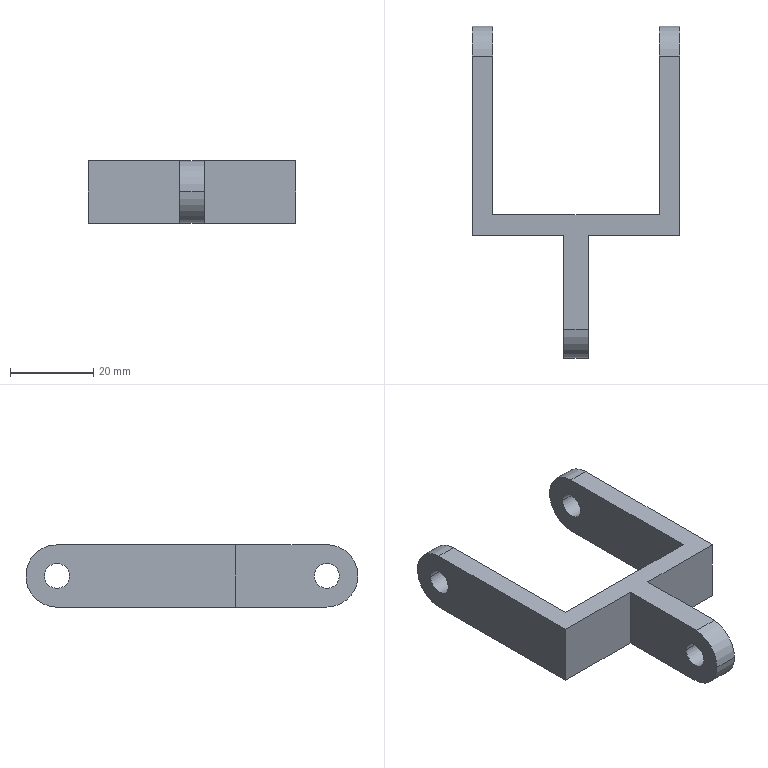Part | SolidWorks | features Extrusion 1, ICE 1 | 1 solid | 24 faces | box 50 x 80 x 15 mm | volume 12391 mm3 | plane 14 | cylinder 10 | commonest cylinder face diameters 6 x6 15 x4
STEP:
#1=CARTESIAN_POINT('',(25.,76.,7.503));
#2=VERTEX_POINT('',#1);
#3=CARTESIAN_POINT('',(25.,70.,7.503));
#4=VERTEX_POINT('',#3);
#5=CARTESIAN_POINT('',(25.,73.,7.503));
#6=DIRECTION('',(-1.,0.,0.));
#7=DIRECTION('',(0.,-1.,0.));
#8=AXIS2_PLACEMENT_3D('',#5,#6,#7);
#9=CIRCLE('',#8,3.);
#10=EDGE_CURVE('',#2,#4,#9,.T.);
#11=ORIENTED_EDGE('',*,*,#10,.F.);
#12=CARTESIAN_POINT('',(20.,76.,7.503));
#13=VERTEX_POINT('',#12);
#14=CARTESIAN_POINT('',(25.,76.,7.503));
#15=DIRECTION('',(-1.,0.,0.));
#16=VECTOR('',#15,1000.);
#17=LINE('',#14,#16);
#18=EDGE_CURVE('',#2,#13,#17,.T.);
#19=ORIENTED_EDGE('',*,*,#18,.T.);
#20=CARTESIAN_POINT('',(20.,70.,7.503));
#21=VERTEX_POINT('',#20);
#22=CARTESIAN_POINT('',(20.,73.,7.503));
#23=DIRECTION('',(1.,0.,0.));
#24=DIRECTION('',(0.,0.,-1.));
#25=AXIS2_PLACEMENT_3D('',#22,#23,#24);
#26=CIRCLE('',#25,3.);
#27=EDGE_CURVE('',#21,#13,#26,.T.);
#28=ORIENTED_EDGE('',*,*,#27,.F.);
#29=CARTESIAN_POINT('',(25.,70.,7.503));
#30=DIRECTION('',(-1.,0.,0.));
#31=VECTOR('',#30,1000.);
#32=LINE('',#29,#31);
#33=EDGE_CURVE('',#4,#21,#32,.T.);
#34=ORIENTED_EDGE('',*,*,#33,.F.);
#35=EDGE_LOOP('',(#11,#19,#28,#34));
#36=FACE_OUTER_BOUND('',#35,.T.);
#37=CARTESIAN_POINT('',(25.,73.,7.503));
#38=DIRECTION('',(-1.,0.,0.));
#39=DIRECTION('',(0.,-1.,0.));
#40=AXIS2_PLACEMENT_3D('',#37,#38,#39);
#41=CYLINDRICAL_SURFACE('',#40,3.);
#42=ADVANCED_FACE('',(#36),#41,.F.);
#43=CARTESIAN_POINT('',(-20.,76.,7.503));
#44=VERTEX_POINT('',#43);
#45=CARTESIAN_POINT('',(-20.,70.,7.503));
#46=VERTEX_POINT('',#45);
#47=CARTESIAN_POINT('',(-20.,73.,7.503));
#48=DIRECTION('',(-1.,0.,0.));
#49=DIRECTION('',(0.,0.,1.));
#50=AXIS2_PLACEMENT_3D('',#47,#48,#49);
#51=CIRCLE('',#50,3.);
#52=EDGE_CURVE('',#44,#46,#51,.T.);
#53=ORIENTED_EDGE('',*,*,#52,.F.);
#54=CARTESIAN_POINT('',(-25.,76.,7.503));
#55=VERTEX_POINT('',#54);
#56=CARTESIAN_POINT('',(25.,76.,7.503));
#57=DIRECTION('',(-1.,0.,0.));
#58=VECTOR('',#57,1000.);
#59=LINE('',#56,#58);
#60=EDGE_CURVE('',#44,#55,#59,.T.);
#61=ORIENTED_EDGE('',*,*,#60,.T.);
#62=CARTESIAN_POINT('',(-25.,70.,7.503));
#63=VERTEX_POINT('',#62);
#64=CARTESIAN_POINT('',(-25.,73.,7.503));
#65=DIRECTION('',(-1.,0.,0.));
#66=DIRECTION('',(0.,-1.,0.));
#67=AXIS2_PLACEMENT_3D('',#64,#65,#66);
#68=CIRCLE('',#67,3.);
#69=EDGE_CURVE('',#55,#63,#68,.T.);
#70=ORIENTED_EDGE('',*,*,#69,.T.);
#71=CARTESIAN_POINT('',(25.,70.,7.503));
#72=DIRECTION('',(-1.,0.,0.));
#73=VECTOR('',#72,1000.);
#74=LINE('',#71,#73);
#75=EDGE_CURVE('',#46,#63,#74,.T.);
#76=ORIENTED_EDGE('',*,*,#75,.F.);
#77=EDGE_LOOP('',(#53,#61,#70,#76));
#78=FACE_OUTER_BOUND('',#77,.T.);
#79=CARTESIAN_POINT('',(25.,73.,7.503));
#80=DIRECTION('',(-1.,0.,0.));
#81=DIRECTION('',(0.,-1.,0.));
#82=AXIS2_PLACEMENT_3D('',#79,#80,#81);
#83=CYLINDRICAL_SURFACE('',#82,3.);
#84=ADVANCED_FACE('',(#78),#83,.F.);
#85=CARTESIAN_POINT('',(3.,11.,7.524));
#86=VERTEX_POINT('',#85);
#87=CARTESIAN_POINT('',(3.,5.,7.524));
#88=VERTEX_POINT('',#87);
#89=CARTESIAN_POINT('',(3.,8.,7.524));
#90=DIRECTION('',(-1.,0.,0.));
#91=DIRECTION('',(0.,-1.,0.));
#92=AXIS2_PLACEMENT_3D('',#89,#90,#91);
#93=CIRCLE('',#92,3.);
#94=EDGE_CURVE('',#86,#88,#93,.T.);
#95=ORIENTED_EDGE('',*,*,#94,.F.);
#96=CARTESIAN_POINT('',(-3.,11.,7.524));
#97=VERTEX_POINT('',#96);
#98=CARTESIAN_POINT('',(25.,11.,7.524));
#99=DIRECTION('',(-1.,0.,0.));
#100=VECTOR('',#99,1000.);
#101=LINE('',#98,#100);
#102=EDGE_CURVE('',#86,#97,#101,.T.);
#103=ORIENTED_EDGE('',*,*,#102,.T.);
#104=CARTESIAN_POINT('',(-3.,5.,7.524));
#105=VERTEX_POINT('',#104);
#106=CARTESIAN_POINT('',(-3.,8.,7.524));
#107=DIRECTION('',(1.,0.,0.));
#108=DIRECTION('',(0.,1.,0.));
#109=AXIS2_PLACEMENT_3D('',#106,#107,#108);
#110=CIRCLE('',#109,3.);
#111=EDGE_CURVE('',#105,#97,#110,.T.);
#112=ORIENTED_EDGE('',*,*,#111,.F.);
#113=CARTESIAN_POINT('',(25.,5.,7.524));
#114=DIRECTION('',(-1.,0.,0.));
#115=VECTOR('',#114,1000.);
#116=LINE('',#113,#115);
#117=EDGE_CURVE('',#88,#105,#116,.T.);
#118=ORIENTED_EDGE('',*,*,#117,.F.);
#119=EDGE_LOOP('',(#95,#103,#112,#118));
#120=FACE_OUTER_BOUND('',#119,.T.);
#121=CARTESIAN_POINT('',(25.,8.,7.524));
#122=DIRECTION('',(-1.,0.,0.));
#123=DIRECTION('',(0.,-1.,0.));
#124=AXIS2_PLACEMENT_3D('',#121,#122,#123);
#125=CYLINDRICAL_SURFACE('',#124,3.);
#126=ADVANCED_FACE('',(#120),#125,.F.);
#127=CARTESIAN_POINT('',(3.,0.5,7.524));
#128=VERTEX_POINT('',#127);
#129=CARTESIAN_POINT('',(3.,8.,0.02363));
#130=VERTEX_POINT('',#129);
#131=CARTESIAN_POINT('',(3.,8.,7.524));
#132=DIRECTION('',(1.,0.,0.));
#133=DIRECTION('',(0.,-1.,0.));
#134=AXIS2_PLACEMENT_3D('',#131,#132,#133);
#135=CIRCLE('',#134,7.5);
#136=EDGE_CURVE('',#128,#130,#135,.T.);
#137=ORIENTED_EDGE('',*,*,#136,.F.);
#138=CARTESIAN_POINT('',(-3.,0.5,7.524));
#139=VERTEX_POINT('',#138);
#140=CARTESIAN_POINT('',(25.,0.5,7.524));
#141=DIRECTION('',(-1.,0.,0.));
#142=VECTOR('',#141,1000.);
#143=LINE('',#140,#142);
#144=EDGE_CURVE('',#128,#139,#143,.T.);
#145=ORIENTED_EDGE('',*,*,#144,.T.);
#146=CARTESIAN_POINT('',(-3.,8.,0.02363));
#147=VERTEX_POINT('',#146);
#148=CARTESIAN_POINT('',(-3.,8.,7.524));
#149=DIRECTION('',(-1.,0.,0.));
#150=DIRECTION('',(0.,1.,0.));
#151=AXIS2_PLACEMENT_3D('',#148,#149,#150);
#152=CIRCLE('',#151,7.5);
#153=EDGE_CURVE('',#147,#139,#152,.T.);
#154=ORIENTED_EDGE('',*,*,#153,.F.);
#155=CARTESIAN_POINT('',(25.,8.,0.02363));
#156=DIRECTION('',(-1.,0.,0.));
#157=VECTOR('',#156,1000.);
#158=LINE('',#155,#157);
#159=EDGE_CURVE('',#130,#147,#158,.T.);
#160=ORIENTED_EDGE('',*,*,#159,.F.);
#161=EDGE_LOOP('',(#137,#145,#154,#160));
#162=FACE_OUTER_BOUND('',#161,.T.);
#163=CARTESIAN_POINT('',(25.,8.,7.524));
#164=DIRECTION('',(-1.,0.,0.));
#165=DIRECTION('',(0.,-1.,0.));
#166=AXIS2_PLACEMENT_3D('',#163,#164,#165);
#167=CYLINDRICAL_SURFACE('',#166,7.5);
#168=ADVANCED_FACE('',(#162),#167,.T.);
#169=CARTESIAN_POINT('',(3.,8.,7.524));
#170=DIRECTION('',(-1.,0.,0.));
#171=DIRECTION('',(0.,-1.,0.));
#172=AXIS2_PLACEMENT_3D('',#169,#170,#171);
#173=CIRCLE('',#172,3.);
#174=EDGE_CURVE('',#88,#86,#173,.T.);
#175=ORIENTED_EDGE('',*,*,#174,.T.);
#176=ORIENTED_EDGE('',*,*,#94,.T.);
#177=EDGE_LOOP('',(#175,#176));
#178=FACE_BOUND('',#177,.T.);
#179=CARTESIAN_POINT('',(3.,7.405,15.));
#180=VERTEX_POINT('',#179);
#181=CARTESIAN_POINT('',(3.,30.,15.));
#182=VERTEX_POINT('',#181);
#183=CARTESIAN_POINT('',(3.,30.,15.));
#184=DIRECTION('',(0.,1.,0.));
#185=VECTOR('',#184,1000.);
#186=LINE('',#183,#185);
#187=EDGE_CURVE('',#180,#182,#186,.T.);
#188=ORIENTED_EDGE('',*,*,#187,.F.);
#189=CARTESIAN_POINT('',(3.,8.,7.524));
#190=DIRECTION('',(1.,0.,0.));
#191=DIRECTION('',(0.,-1.,0.));
#192=AXIS2_PLACEMENT_3D('',#189,#190,#191);
#193=CIRCLE('',#192,7.5);
#194=EDGE_CURVE('',#180,#128,#193,.T.);
#195=ORIENTED_EDGE('',*,*,#194,.T.);
#196=ORIENTED_EDGE('',*,*,#136,.T.);
#197=CARTESIAN_POINT('',(3.,7.989,0.));
#198=VERTEX_POINT('',#197);
#199=CARTESIAN_POINT('',(3.,18.014,20.782));
#200=DIRECTION('',(0.,-0.4345,-0.9007));
#201=VECTOR('',#200,1000.);
#202=LINE('',#199,#201);
#203=EDGE_CURVE('',#130,#198,#202,.T.);
#204=ORIENTED_EDGE('',*,*,#203,.T.);
#205=CARTESIAN_POINT('',(3.,30.,0.));
#206=VERTEX_POINT('',#205);
#207=CARTESIAN_POINT('',(3.,30.,0.));
#208=DIRECTION('',(0.,1.,0.));
#209=VECTOR('',#208,1000.);
#210=LINE('',#207,#209);
#211=EDGE_CURVE('',#198,#206,#210,.T.);
#212=ORIENTED_EDGE('',*,*,#211,.T.);
#213=CARTESIAN_POINT('',(3.,30.,15.));
#214=DIRECTION('',(0.,0.,-1.));
#215=VECTOR('',#214,1000.);
#216=LINE('',#213,#215);
#217=EDGE_CURVE('',#182,#206,#216,.T.);
#218=ORIENTED_EDGE('',*,*,#217,.F.);
#219=EDGE_LOOP('',(#188,#195,#196,#204,#212,#218));
#220=FACE_OUTER_BOUND('',#219,.T.);
#221=CARTESIAN_POINT('',(3.,30.,15.));
#222=DIRECTION('',(-1.,0.,0.));
#223=DIRECTION('',(0.,-1.,0.));
#224=AXIS2_PLACEMENT_3D('',#221,#222,#223);
#225=PLANE('',#224);
#226=ADVANCED_FACE('',(#178,#220),#225,.F.);
#227=CARTESIAN_POINT('',(25.,30.,0.));
#228=VERTEX_POINT('',#227);
#229=CARTESIAN_POINT('',(25.,30.,0.));
#230=DIRECTION('',(1.,0.,0.));
#231=VECTOR('',#230,1000.);
#232=LINE('',#229,#231);
#233=EDGE_CURVE('',#206,#228,#232,.T.);
#234=ORIENTED_EDGE('',*,*,#233,.T.);
#235=CARTESIAN_POINT('',(25.,30.,15.));
#236=VERTEX_POINT('',#235);
#237=CARTESIAN_POINT('',(25.,30.,15.));
#238=DIRECTION('',(0.,0.,-1.));
#239=VECTOR('',#238,1000.);
#240=LINE('',#237,#239);
#241=EDGE_CURVE('',#236,#228,#240,.T.);
#242=ORIENTED_EDGE('',*,*,#241,.F.);
#243=CARTESIAN_POINT('',(25.,30.,15.));
#244=DIRECTION('',(1.,0.,0.));
#245=VECTOR('',#244,1000.);
#246=LINE('',#243,#245);
#247=EDGE_CURVE('',#182,#236,#246,.T.);
#248=ORIENTED_EDGE('',*,*,#247,.F.);
#249=ORIENTED_EDGE('',*,*,#217,.T.);
#250=EDGE_LOOP('',(#234,#242,#248,#249));
#251=FACE_OUTER_BOUND('',#250,.T.);
#252=CARTESIAN_POINT('',(25.,30.,15.));
#253=DIRECTION('',(0.,1.,0.));
#254=DIRECTION('',(0.,0.,1.));
#255=AXIS2_PLACEMENT_3D('',#252,#253,#254);
#256=PLANE('',#255);
#257=ADVANCED_FACE('',(#251),#256,.F.);
#258=CARTESIAN_POINT('',(25.,73.,7.503));
#259=DIRECTION('',(-1.,0.,0.));
#260=DIRECTION('',(0.,-1.,0.));
#261=AXIS2_PLACEMENT_3D('',#258,#259,#260);
#262=CIRCLE('',#261,3.);
#263=EDGE_CURVE('',#4,#2,#262,.T.);
#264=ORIENTED_EDGE('',*,*,#263,.T.);
#265=ORIENTED_EDGE('',*,*,#10,.T.);
#266=EDGE_LOOP('',(#264,#265));
#267=FACE_BOUND('',#266,.T.);
#268=CARTESIAN_POINT('',(25.,73.001,0.));
#269=VERTEX_POINT('',#268);
#270=CARTESIAN_POINT('',(25.,73.,0.00323));
#271=VERTEX_POINT('',#270);
#272=CARTESIAN_POINT('',(25.,73.,0.00323));
#273=DIRECTION('',(0.,-0.159,0.9873));
#274=VECTOR('',#273,1000.);
#275=LINE('',#272,#274);
#276=EDGE_CURVE('',#269,#271,#275,.T.);
#277=ORIENTED_EDGE('',*,*,#276,.T.);
#278=CARTESIAN_POINT('',(25.,73.22,15.));
#279=VERTEX_POINT('',#278);
#280=CARTESIAN_POINT('',(25.,73.,7.503));
#281=DIRECTION('',(1.,0.,0.));
#282=DIRECTION('',(0.,-1.,0.));
#283=AXIS2_PLACEMENT_3D('',#280,#281,#282);
#284=CIRCLE('',#283,7.5);
#285=EDGE_CURVE('',#271,#279,#284,.T.);
#286=ORIENTED_EDGE('',*,*,#285,.T.);
#287=CARTESIAN_POINT('',(25.,85.,15.));
#288=DIRECTION('',(0.,1.,0.));
#289=VECTOR('',#288,1000.);
#290=LINE('',#287,#289);
#291=EDGE_CURVE('',#236,#279,#290,.T.);
#292=ORIENTED_EDGE('',*,*,#291,.F.);
#293=ORIENTED_EDGE('',*,*,#241,.T.);
#294=CARTESIAN_POINT('',(25.,85.,0.));
#295=DIRECTION('',(0.,1.,0.));
#296=VECTOR('',#295,1000.);
#297=LINE('',#294,#296);
#298=EDGE_CURVE('',#228,#269,#297,.T.);
#299=ORIENTED_EDGE('',*,*,#298,.T.);
#300=EDGE_LOOP('',(#277,#286,#292,#293,#299));
#301=FACE_OUTER_BOUND('',#300,.T.);
#302=CARTESIAN_POINT('',(25.,85.,15.));
#303=DIRECTION('',(-1.,0.,0.));
#304=DIRECTION('',(0.,-1.,0.));
#305=AXIS2_PLACEMENT_3D('',#302,#303,#304);
#306=PLANE('',#305);
#307=ADVANCED_FACE('',(#267,#301),#306,.F.);
#308=ORIENTED_EDGE('',*,*,#27,.T.);
#309=CARTESIAN_POINT('',(20.,73.,7.503));
#310=DIRECTION('',(1.,0.,0.));
#311=DIRECTION('',(0.,0.,-1.));
#312=AXIS2_PLACEMENT_3D('',#309,#310,#311);
#313=CIRCLE('',#312,3.);
#314=EDGE_CURVE('',#13,#21,#313,.T.);
#315=ORIENTED_EDGE('',*,*,#314,.T.);
#316=EDGE_LOOP('',(#308,#315));
#317=FACE_BOUND('',#316,.T.);
#318=CARTESIAN_POINT('',(20.,73.22,15.));
#319=VERTEX_POINT('',#318);
#320=CARTESIAN_POINT('',(20.,35.,15.));
#321=VERTEX_POINT('',#320);
#322=CARTESIAN_POINT('',(20.,35.,15.));
#323=DIRECTION('',(0.,-1.,0.));
#324=VECTOR('',#323,1000.);
#325=LINE('',#322,#324);
#326=EDGE_CURVE('',#319,#321,#325,.T.);
#327=ORIENTED_EDGE('',*,*,#326,.F.);
#328=CARTESIAN_POINT('',(20.,73.,0.00323));
#329=VERTEX_POINT('',#328);
#330=CARTESIAN_POINT('',(20.,73.,7.503));
#331=DIRECTION('',(-1.,0.,0.));
#332=DIRECTION('',(0.,0.,-1.));
#333=AXIS2_PLACEMENT_3D('',#330,#331,#332);
#334=CIRCLE('',#333,7.5);
#335=EDGE_CURVE('',#319,#329,#334,.T.);
#336=ORIENTED_EDGE('',*,*,#335,.T.);
#337=CARTESIAN_POINT('',(20.,73.001,0.));
#338=VERTEX_POINT('',#337);
#339=CARTESIAN_POINT('',(20.,69.684,20.587));
#340=DIRECTION('',(0.,0.159,-0.9873));
#341=VECTOR('',#340,1000.);
#342=LINE('',#339,#341);
#343=EDGE_CURVE('',#329,#338,#342,.T.);
#344=ORIENTED_EDGE('',*,*,#343,.T.);
#345=CARTESIAN_POINT('',(20.,35.,0.));
#346=VERTEX_POINT('',#345);
#347=CARTESIAN_POINT('',(20.,35.,0.));
#348=DIRECTION('',(0.,-1.,0.));
#349=VECTOR('',#348,1000.);
#350=LINE('',#347,#349);
#351=EDGE_CURVE('',#338,#346,#350,.T.);
#352=ORIENTED_EDGE('',*,*,#351,.T.);
#353=CARTESIAN_POINT('',(20.,35.,15.));
#354=DIRECTION('',(0.,0.,-1.));
#355=VECTOR('',#354,1000.);
#356=LINE('',#353,#355);
#357=EDGE_CURVE('',#321,#346,#356,.T.);
#358=ORIENTED_EDGE('',*,*,#357,.F.);
#359=EDGE_LOOP('',(#327,#336,#344,#352,#358));
#360=FACE_OUTER_BOUND('',#359,.T.);
#361=CARTESIAN_POINT('',(20.,35.,15.));
#362=DIRECTION('',(1.,0.,0.));
#363=DIRECTION('',(0.,0.,-1.));
#364=AXIS2_PLACEMENT_3D('',#361,#362,#363);
#365=PLANE('',#364);
#366=ADVANCED_FACE('',(#317,#360),#365,.F.);
#367=CARTESIAN_POINT('',(-20.,35.,0.));
#368=VERTEX_POINT('',#367);
#369=CARTESIAN_POINT('',(20.,35.,0.));
#370=DIRECTION('',(-1.,0.,0.));
#371=VECTOR('',#370,1000.);
#372=LINE('',#369,#371);
#373=EDGE_CURVE('',#346,#368,#372,.T.);
#374=ORIENTED_EDGE('',*,*,#373,.T.);
#375=CARTESIAN_POINT('',(-20.,35.,15.));
#376=VERTEX_POINT('',#375);
#377=CARTESIAN_POINT('',(-20.,35.,15.));
#378=DIRECTION('',(0.,0.,-1.));
#379=VECTOR('',#378,1000.);
#380=LINE('',#377,#379);
#381=EDGE_CURVE('',#376,#368,#380,.T.);
#382=ORIENTED_EDGE('',*,*,#381,.F.);
#383=CARTESIAN_POINT('',(20.,35.,15.));
#384=DIRECTION('',(-1.,0.,0.));
#385=VECTOR('',#384,1000.);
#386=LINE('',#383,#385);
#387=EDGE_CURVE('',#321,#376,#386,.T.);
#388=ORIENTED_EDGE('',*,*,#387,.F.);
#389=ORIENTED_EDGE('',*,*,#357,.T.);
#390=EDGE_LOOP('',(#374,#382,#388,#389));
#391=FACE_OUTER_BOUND('',#390,.T.);
#392=CARTESIAN_POINT('',(20.,35.,15.));
#393=DIRECTION('',(0.,-1.,0.));
#394=DIRECTION('',(0.,0.,-1.));
#395=AXIS2_PLACEMENT_3D('',#392,#393,#394);
#396=PLANE('',#395);
#397=ADVANCED_FACE('',(#391),#396,.F.);
#398=CARTESIAN_POINT('',(-20.,73.,7.503));
#399=DIRECTION('',(-1.,0.,0.));
#400=DIRECTION('',(0.,0.,1.));
#401=AXIS2_PLACEMENT_3D('',#398,#399,#400);
#402=CIRCLE('',#401,3.);
#403=EDGE_CURVE('',#46,#44,#402,.T.);
#404=ORIENTED_EDGE('',*,*,#403,.T.);
#405=ORIENTED_EDGE('',*,*,#52,.T.);
#406=EDGE_LOOP('',(#404,#405));
#407=FACE_BOUND('',#406,.T.);
#408=CARTESIAN_POINT('',(-20.,73.001,0.));
#409=VERTEX_POINT('',#408);
#410=CARTESIAN_POINT('',(-20.,73.,0.00323));
#411=VERTEX_POINT('',#410);
#412=CARTESIAN_POINT('',(-20.,69.684,20.587));
#413=DIRECTION('',(0.,-0.159,0.9873));
#414=VECTOR('',#413,1000.);
#415=LINE('',#412,#414);
#416=EDGE_CURVE('',#409,#411,#415,.T.);
#417=ORIENTED_EDGE('',*,*,#416,.T.);
#418=CARTESIAN_POINT('',(-20.,73.22,15.));
#419=VERTEX_POINT('',#418);
#420=CARTESIAN_POINT('',(-20.,73.,7.503));
#421=DIRECTION('',(1.,0.,0.));
#422=DIRECTION('',(0.,0.,1.));
#423=AXIS2_PLACEMENT_3D('',#420,#421,#422);
#424=CIRCLE('',#423,7.5);
#425=EDGE_CURVE('',#411,#419,#424,.T.);
#426=ORIENTED_EDGE('',*,*,#425,.T.);
#427=CARTESIAN_POINT('',(-20.,35.,15.));
#428=DIRECTION('',(0.,1.,0.));
#429=VECTOR('',#428,1000.);
#430=LINE('',#427,#429);
#431=EDGE_CURVE('',#376,#419,#430,.T.);
#432=ORIENTED_EDGE('',*,*,#431,.F.);
#433=ORIENTED_EDGE('',*,*,#381,.T.);
#434=CARTESIAN_POINT('',(-20.,35.,0.));
#435=DIRECTION('',(0.,1.,0.));
#436=VECTOR('',#435,1000.);
#437=LINE('',#434,#436);
#438=EDGE_CURVE('',#368,#409,#437,.T.);
#439=ORIENTED_EDGE('',*,*,#438,.T.);
#440=EDGE_LOOP('',(#417,#426,#432,#433,#439));
#441=FACE_OUTER_BOUND('',#440,.T.);
#442=CARTESIAN_POINT('',(-20.,35.,15.));
#443=DIRECTION('',(-1.,0.,0.));
#444=DIRECTION('',(0.,0.,1.));
#445=AXIS2_PLACEMENT_3D('',#442,#443,#444);
#446=PLANE('',#445);
#447=ADVANCED_FACE('',(#407,#441),#446,.F.);
#448=CARTESIAN_POINT('',(-25.,73.,7.503));
#449=DIRECTION('',(-1.,0.,0.));
#450=DIRECTION('',(0.,-1.,0.));
#451=AXIS2_PLACEMENT_3D('',#448,#449,#450);
#452=CIRCLE('',#451,3.);
#453=EDGE_CURVE('',#63,#55,#452,.T.);
#454=ORIENTED_EDGE('',*,*,#453,.F.);
#455=ORIENTED_EDGE('',*,*,#69,.F.);
#456=EDGE_LOOP('',(#454,#455));
#457=FACE_BOUND('',#456,.T.);
#458=CARTESIAN_POINT('',(-25.,73.22,15.));
#459=VERTEX_POINT('',#458);
#460=CARTESIAN_POINT('',(-25.,30.,15.));
#461=VERTEX_POINT('',#460);
#462=CARTESIAN_POINT('',(-25.,85.,15.));
#463=DIRECTION('',(0.,-1.,0.));
#464=VECTOR('',#463,1000.);
#465=LINE('',#462,#464);
#466=EDGE_CURVE('',#459,#461,#465,.T.);
#467=ORIENTED_EDGE('',*,*,#466,.F.);
#468=CARTESIAN_POINT('',(-25.,73.,0.00323));
#469=VERTEX_POINT('',#468);
#470=CARTESIAN_POINT('',(-25.,73.,7.503));
#471=DIRECTION('',(1.,0.,0.));
#472=DIRECTION('',(0.,-1.,0.));
#473=AXIS2_PLACEMENT_3D('',#470,#471,#472);
#474=CIRCLE('',#473,7.5);
#475=EDGE_CURVE('',#469,#459,#474,.T.);
#476=ORIENTED_EDGE('',*,*,#475,.F.);
#477=CARTESIAN_POINT('',(-25.,73.001,0.));
#478=VERTEX_POINT('',#477);
#479=CARTESIAN_POINT('',(-25.,73.,0.00323));
#480=DIRECTION('',(0.,-0.159,0.9873));
#481=VECTOR('',#480,1000.);
#482=LINE('',#479,#481);
#483=EDGE_CURVE('',#478,#469,#482,.T.);
#484=ORIENTED_EDGE('',*,*,#483,.F.);
#485=CARTESIAN_POINT('',(-25.,30.,0.));
#486=VERTEX_POINT('',#485);
#487=CARTESIAN_POINT('',(-25.,85.,0.));
#488=DIRECTION('',(0.,-1.,0.));
#489=VECTOR('',#488,1000.);
#490=LINE('',#487,#489);
#491=EDGE_CURVE('',#478,#486,#490,.T.);
#492=ORIENTED_EDGE('',*,*,#491,.T.);
#493=CARTESIAN_POINT('',(-25.,30.,15.));
#494=DIRECTION('',(0.,0.,-1.));
#495=VECTOR('',#494,1000.);
#496=LINE('',#493,#495);
#497=EDGE_CURVE('',#461,#486,#496,.T.);
#498=ORIENTED_EDGE('',*,*,#497,.F.);
#499=EDGE_LOOP('',(#467,#476,#484,#492,#498));
#500=FACE_OUTER_BOUND('',#499,.T.);
#501=CARTESIAN_POINT('',(-25.,85.,15.));
#502=DIRECTION('',(1.,0.,0.));
#503=DIRECTION('',(0.,1.,0.));
#504=AXIS2_PLACEMENT_3D('',#501,#502,#503);
#505=PLANE('',#504);
#506=ADVANCED_FACE('',(#457,#500),#505,.F.);
#507=CARTESIAN_POINT('',(-3.,30.,0.));
#508=VERTEX_POINT('',#507);
#509=CARTESIAN_POINT('',(-25.,30.,0.));
#510=DIRECTION('',(1.,0.,0.));
#511=VECTOR('',#510,1000.);
#512=LINE('',#509,#511);
#513=EDGE_CURVE('',#486,#508,#512,.T.);
#514=ORIENTED_EDGE('',*,*,#513,.T.);
#515=CARTESIAN_POINT('',(-3.,30.,15.));
#516=VERTEX_POINT('',#515);
#517=CARTESIAN_POINT('',(-3.,30.,15.));
#518=DIRECTION('',(0.,0.,-1.));
#519=VECTOR('',#518,1000.);
#520=LINE('',#517,#519);
#521=EDGE_CURVE('',#516,#508,#520,.T.);
#522=ORIENTED_EDGE('',*,*,#521,.F.);
#523=CARTESIAN_POINT('',(-25.,30.,15.));
#524=DIRECTION('',(1.,0.,0.));
#525=VECTOR('',#524,1000.);
#526=LINE('',#523,#525);
#527=EDGE_CURVE('',#461,#516,#526,.T.);
#528=ORIENTED_EDGE('',*,*,#527,.F.);
#529=ORIENTED_EDGE('',*,*,#497,.T.);
#530=EDGE_LOOP('',(#514,#522,#528,#529));
#531=FACE_OUTER_BOUND('',#530,.T.);
#532=CARTESIAN_POINT('',(-25.,30.,15.));
#533=DIRECTION('',(0.,1.,0.));
#534=DIRECTION('',(0.,0.,1.));
#535=AXIS2_PLACEMENT_3D('',#532,#533,#534);
#536=PLANE('',#535);
#537=ADVANCED_FACE('',(#531),#536,.F.);
#538=ORIENTED_EDGE('',*,*,#111,.T.);
#539=CARTESIAN_POINT('',(-3.,8.,7.524));
#540=DIRECTION('',(1.,0.,0.));
#541=DIRECTION('',(0.,1.,0.));
#542=AXIS2_PLACEMENT_3D('',#539,#540,#541);
#543=CIRCLE('',#542,3.);
#544=EDGE_CURVE('',#97,#105,#543,.T.);
#545=ORIENTED_EDGE('',*,*,#544,.T.);
#546=EDGE_LOOP('',(#538,#545));
#547=FACE_BOUND('',#546,.T.);
#548=CARTESIAN_POINT('',(-3.,7.989,0.));
#549=VERTEX_POINT('',#548);
#550=CARTESIAN_POINT('',(-3.,18.014,20.782));
#551=DIRECTION('',(0.,0.4345,0.9007));
#552=VECTOR('',#551,1000.);
#553=LINE('',#550,#552);
#554=EDGE_CURVE('',#549,#147,#553,.T.);
#555=ORIENTED_EDGE('',*,*,#554,.T.);
#556=ORIENTED_EDGE('',*,*,#153,.T.);
#557=CARTESIAN_POINT('',(-3.,7.405,15.));
#558=VERTEX_POINT('',#557);
#559=CARTESIAN_POINT('',(-3.,8.,7.524));
#560=DIRECTION('',(-1.,0.,0.));
#561=DIRECTION('',(0.,1.,0.));
#562=AXIS2_PLACEMENT_3D('',#559,#560,#561);
#563=CIRCLE('',#562,7.5);
#564=EDGE_CURVE('',#139,#558,#563,.T.);
#565=ORIENTED_EDGE('',*,*,#564,.T.);
#566=CARTESIAN_POINT('',(-3.,30.,15.));
#567=DIRECTION('',(0.,-1.,0.));
#568=VECTOR('',#567,1000.);
#569=LINE('',#566,#568);
#570=EDGE_CURVE('',#516,#558,#569,.T.);
#571=ORIENTED_EDGE('',*,*,#570,.F.);
#572=ORIENTED_EDGE('',*,*,#521,.T.);
#573=CARTESIAN_POINT('',(-3.,30.,0.));
#574=DIRECTION('',(0.,-1.,0.));
#575=VECTOR('',#574,1000.);
#576=LINE('',#573,#575);
#577=EDGE_CURVE('',#508,#549,#576,.T.);
#578=ORIENTED_EDGE('',*,*,#577,.T.);
#579=EDGE_LOOP('',(#555,#556,#565,#571,#572,#578));
#580=FACE_OUTER_BOUND('',#579,.T.);
#581=CARTESIAN_POINT('',(-3.,30.,15.));
#582=DIRECTION('',(1.,0.,0.));
#583=DIRECTION('',(0.,1.,0.));
#584=AXIS2_PLACEMENT_3D('',#581,#582,#583);
#585=PLANE('',#584);
#586=ADVANCED_FACE('',(#547,#580),#585,.F.);
#587=ORIENTED_EDGE('',*,*,#291,.T.);
#588=CARTESIAN_POINT('',(25.,73.22,15.));
#589=DIRECTION('',(-1.,0.,0.));
#590=VECTOR('',#589,1000.);
#591=LINE('',#588,#590);
#592=EDGE_CURVE('',#279,#319,#591,.T.);
#593=ORIENTED_EDGE('',*,*,#592,.T.);
#594=ORIENTED_EDGE('',*,*,#326,.T.);
#595=ORIENTED_EDGE('',*,*,#387,.T.);
#596=ORIENTED_EDGE('',*,*,#431,.T.);
#597=CARTESIAN_POINT('',(25.,73.22,15.));
#598=DIRECTION('',(-1.,0.,0.));
#599=VECTOR('',#598,1000.);
#600=LINE('',#597,#599);
#601=EDGE_CURVE('',#419,#459,#600,.T.);
#602=ORIENTED_EDGE('',*,*,#601,.T.);
#603=ORIENTED_EDGE('',*,*,#466,.T.);
#604=ORIENTED_EDGE('',*,*,#527,.T.);
#605=ORIENTED_EDGE('',*,*,#570,.T.);
#606=CARTESIAN_POINT('',(25.,7.405,15.));
#607=DIRECTION('',(1.,0.,0.));
#608=VECTOR('',#607,1000.);
#609=LINE('',#606,#608);
#610=EDGE_CURVE('',#558,#180,#609,.T.);
#611=ORIENTED_EDGE('',*,*,#610,.T.);
#612=ORIENTED_EDGE('',*,*,#187,.T.);
#613=ORIENTED_EDGE('',*,*,#247,.T.);
#614=EDGE_LOOP('',(#587,#593,#594,#595,#596,#602,#603,#604,#605,#611,#612,#613));
#615=FACE_OUTER_BOUND('',#614,.T.);
#616=CARTESIAN_POINT('',(0.,0.,15.));
#617=DIRECTION('',(0.,0.,-1.));
#618=DIRECTION('',(-1.,0.,0.));
#619=AXIS2_PLACEMENT_3D('',#616,#617,#618);
#620=PLANE('',#619);
#621=ADVANCED_FACE('',(#615),#620,.F.);
#622=CARTESIAN_POINT('',(0.,73.001,0.));
#623=DIRECTION('',(-1.,0.,0.));
#624=VECTOR('',#623,1000.);
#625=LINE('',#622,#624);
#626=EDGE_CURVE('',#269,#338,#625,.T.);
#627=ORIENTED_EDGE('',*,*,#626,.F.);
#628=ORIENTED_EDGE('',*,*,#298,.F.);
#629=ORIENTED_EDGE('',*,*,#233,.F.);
#630=ORIENTED_EDGE('',*,*,#211,.F.);
#631=CARTESIAN_POINT('',(0.,7.989,0.));
#632=DIRECTION('',(1.,0.,0.));
#633=VECTOR('',#632,1000.);
#634=LINE('',#631,#633);
#635=EDGE_CURVE('',#549,#198,#634,.T.);
#636=ORIENTED_EDGE('',*,*,#635,.F.);
#637=ORIENTED_EDGE('',*,*,#577,.F.);
#638=ORIENTED_EDGE('',*,*,#513,.F.);
#639=ORIENTED_EDGE('',*,*,#491,.F.);
#640=CARTESIAN_POINT('',(0.,73.001,0.));
#641=DIRECTION('',(-1.,0.,0.));
#642=VECTOR('',#641,1000.);
#643=LINE('',#640,#642);
#644=EDGE_CURVE('',#409,#478,#643,.T.);
#645=ORIENTED_EDGE('',*,*,#644,.F.);
#646=ORIENTED_EDGE('',*,*,#438,.F.);
#647=ORIENTED_EDGE('',*,*,#373,.F.);
#648=ORIENTED_EDGE('',*,*,#351,.F.);
#649=EDGE_LOOP('',(#627,#628,#629,#630,#636,#637,#638,#639,#645,#646,#647,#648));
#650=FACE_OUTER_BOUND('',#649,.T.);
#651=CARTESIAN_POINT('',(0.,0.,0.));
#652=DIRECTION('',(0.,0.,-1.));
#653=DIRECTION('',(-1.,0.,0.));
#654=AXIS2_PLACEMENT_3D('',#651,#652,#653);
#655=PLANE('',#654);
#656=ADVANCED_FACE('',(#650),#655,.T.);
#657=ORIENTED_EDGE('',*,*,#144,.F.);
#658=ORIENTED_EDGE('',*,*,#194,.F.);
#659=ORIENTED_EDGE('',*,*,#610,.F.);
#660=ORIENTED_EDGE('',*,*,#564,.F.);
#661=EDGE_LOOP('',(#657,#658,#659,#660));
#662=FACE_OUTER_BOUND('',#661,.T.);
#663=CARTESIAN_POINT('',(25.,8.,7.524));
#664=DIRECTION('',(-1.,0.,0.));
#665=DIRECTION('',(0.,-1.,0.));
#666=AXIS2_PLACEMENT_3D('',#663,#664,#665);
#667=CYLINDRICAL_SURFACE('',#666,7.5);
#668=ADVANCED_FACE('',(#662),#667,.T.);
#669=ORIENTED_EDGE('',*,*,#159,.T.);
#670=ORIENTED_EDGE('',*,*,#554,.F.);
#671=ORIENTED_EDGE('',*,*,#635,.T.);
#672=ORIENTED_EDGE('',*,*,#203,.F.);
#673=EDGE_LOOP('',(#669,#670,#671,#672));
#674=FACE_OUTER_BOUND('',#673,.T.);
#675=CARTESIAN_POINT('',(25.,8.,0.02363));
#676=DIRECTION('',(0.,0.9007,-0.4345));
#677=DIRECTION('',(0.,0.4345,0.9007));
#678=AXIS2_PLACEMENT_3D('',#675,#676,#677);
#679=PLANE('',#678);
#680=ADVANCED_FACE('',(#674),#679,.F.);
#681=ORIENTED_EDGE('',*,*,#644,.T.);
#682=ORIENTED_EDGE('',*,*,#483,.T.);
#683=CARTESIAN_POINT('',(25.,73.,0.00323));
#684=DIRECTION('',(-1.,0.,0.));
#685=VECTOR('',#684,1000.);
#686=LINE('',#683,#685);
#687=EDGE_CURVE('',#411,#469,#686,.T.);
#688=ORIENTED_EDGE('',*,*,#687,.F.);
#689=ORIENTED_EDGE('',*,*,#416,.F.);
#690=EDGE_LOOP('',(#681,#682,#688,#689));
#691=FACE_OUTER_BOUND('',#690,.T.);
#692=CARTESIAN_POINT('',(25.,73.,0.00323));
#693=DIRECTION('',(0.,-0.9873,-0.159));
#694=DIRECTION('',(0.,0.159,-0.9873));
#695=AXIS2_PLACEMENT_3D('',#692,#693,#694);
#696=PLANE('',#695);
#697=ADVANCED_FACE('',(#691),#696,.F.);
#698=ORIENTED_EDGE('',*,*,#687,.T.);
#699=ORIENTED_EDGE('',*,*,#475,.T.);
#700=ORIENTED_EDGE('',*,*,#601,.F.);
#701=ORIENTED_EDGE('',*,*,#425,.F.);
#702=EDGE_LOOP('',(#698,#699,#700,#701));
#703=FACE_OUTER_BOUND('',#702,.T.);
#704=CARTESIAN_POINT('',(25.,73.,7.503));
#705=DIRECTION('',(-1.,0.,0.));
#706=DIRECTION('',(0.,-1.,0.));
#707=AXIS2_PLACEMENT_3D('',#704,#705,#706);
#708=CYLINDRICAL_SURFACE('',#707,7.5);
#709=ADVANCED_FACE('',(#703),#708,.T.);
#710=ORIENTED_EDGE('',*,*,#592,.F.);
#711=ORIENTED_EDGE('',*,*,#285,.F.);
#712=CARTESIAN_POINT('',(25.,73.,0.00323));
#713=DIRECTION('',(-1.,0.,0.));
#714=VECTOR('',#713,1000.);
#715=LINE('',#712,#714);
#716=EDGE_CURVE('',#271,#329,#715,.T.);
#717=ORIENTED_EDGE('',*,*,#716,.T.);
#718=ORIENTED_EDGE('',*,*,#335,.F.);
#719=EDGE_LOOP('',(#710,#711,#717,#718));
#720=FACE_OUTER_BOUND('',#719,.T.);
#721=CARTESIAN_POINT('',(25.,73.,7.503));
#722=DIRECTION('',(-1.,0.,0.));
#723=DIRECTION('',(0.,-1.,0.));
#724=AXIS2_PLACEMENT_3D('',#721,#722,#723);
#725=CYLINDRICAL_SURFACE('',#724,7.5);
#726=ADVANCED_FACE('',(#720),#725,.T.);
#727=ORIENTED_EDGE('',*,*,#716,.F.);
#728=ORIENTED_EDGE('',*,*,#276,.F.);
#729=ORIENTED_EDGE('',*,*,#626,.T.);
#730=ORIENTED_EDGE('',*,*,#343,.F.);
#731=EDGE_LOOP('',(#727,#728,#729,#730));
#732=FACE_OUTER_BOUND('',#731,.T.);
#733=CARTESIAN_POINT('',(25.,73.,0.00323));
#734=DIRECTION('',(0.,-0.9873,-0.159));
#735=DIRECTION('',(0.,0.159,-0.9873));
#736=AXIS2_PLACEMENT_3D('',#733,#734,#735);
#737=PLANE('',#736);
#738=ADVANCED_FACE('',(#732),#737,.F.);
#739=ORIENTED_EDGE('',*,*,#102,.F.);
#740=ORIENTED_EDGE('',*,*,#174,.F.);
#741=ORIENTED_EDGE('',*,*,#117,.T.);
#742=ORIENTED_EDGE('',*,*,#544,.F.);
#743=EDGE_LOOP('',(#739,#740,#741,#742));
#744=FACE_OUTER_BOUND('',#743,.T.);
#745=CARTESIAN_POINT('',(25.,8.,7.524));
#746=DIRECTION('',(-1.,0.,0.));
#747=DIRECTION('',(0.,-1.,0.));
#748=AXIS2_PLACEMENT_3D('',#745,#746,#747);
#749=CYLINDRICAL_SURFACE('',#748,3.);
#750=ADVANCED_FACE('',(#744),#749,.F.);
#751=ORIENTED_EDGE('',*,*,#60,.F.);
#752=ORIENTED_EDGE('',*,*,#403,.F.);
#753=ORIENTED_EDGE('',*,*,#75,.T.);
#754=ORIENTED_EDGE('',*,*,#453,.T.);
#755=EDGE_LOOP('',(#751,#752,#753,#754));
#756=FACE_OUTER_BOUND('',#755,.T.);
#757=CARTESIAN_POINT('',(25.,73.,7.503));
#758=DIRECTION('',(-1.,0.,0.));
#759=DIRECTION('',(0.,-1.,0.));
#760=AXIS2_PLACEMENT_3D('',#757,#758,#759);
#761=CYLINDRICAL_SURFACE('',#760,3.);
#762=ADVANCED_FACE('',(#756),#761,.F.);
#763=ORIENTED_EDGE('',*,*,#18,.F.);
#764=ORIENTED_EDGE('',*,*,#263,.F.);
#765=ORIENTED_EDGE('',*,*,#33,.T.);
#766=ORIENTED_EDGE('',*,*,#314,.F.);
#767=EDGE_LOOP('',(#763,#764,#765,#766));
#768=FACE_OUTER_BOUND('',#767,.T.);
#769=CARTESIAN_POINT('',(25.,73.,7.503));
#770=DIRECTION('',(-1.,0.,0.));
#771=DIRECTION('',(0.,-1.,0.));
#772=AXIS2_PLACEMENT_3D('',#769,#770,#771);
#773=CYLINDRICAL_SURFACE('',#772,3.);
#774=ADVANCED_FACE('',(#768),#773,.F.);
#775=CLOSED_SHELL('',(#42,#84,#126,#168,#226,#257,#307,#366,#397,#447,#506,#537,#586,#621,#656,#668,#680,#697,#709,#726,#738,#750,#762,#774));
#776=MANIFOLD_SOLID_BREP('',#775);
#777=CARTESIAN_POINT('',(0.,0.,0.));
#778=DIRECTION('',(0.,0.,1.));
#779=DIRECTION('',(1.,0.,0.));
#780=AXIS2_PLACEMENT_3D('',#777,#778,#779);
#781=(LENGTH_UNIT()NAMED_UNIT(*)SI_UNIT(.MILLI.,.METRE.));
#782=UNCERTAINTY_MEASURE_WITH_UNIT(LENGTH_MEASURE(0.00001),#781,'','');
#783=(NAMED_UNIT(*)PLANE_ANGLE_UNIT()SI_UNIT($,.RADIAN.));
#784=(NAMED_UNIT(*)SI_UNIT($,.STERADIAN.)SOLID_ANGLE_UNIT());
#785=(GEOMETRIC_REPRESENTATION_CONTEXT(3)GLOBAL_UNCERTAINTY_ASSIGNED_CONTEXT((#782))GLOBAL_UNIT_ASSIGNED_CONTEXT((#781,#783,#784))REPRESENTATION_CONTEXT('',''));
#786=ADVANCED_BREP_SHAPE_REPRESENTATION('',(#776,#780),#785);